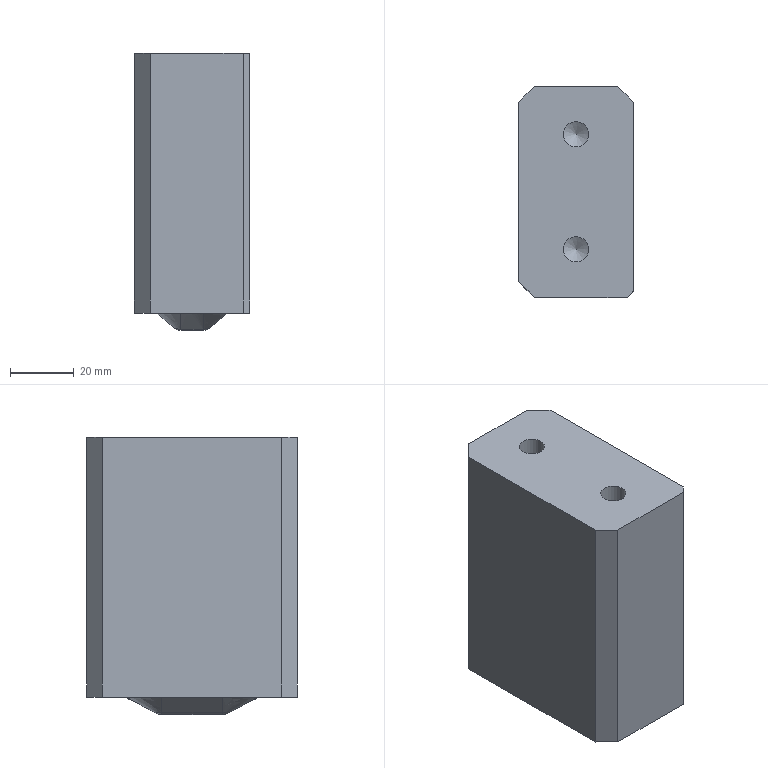Part | STEP file | 1_id138_x_t | 1 solid | 31 faces | box 36 x 66 x 86.679 mm | volume 191132 mm3 | plane 13 | spline 12 | cylinder 4 | cone 2 | commonest cylinder face diameters 6 x2 7.938 x2